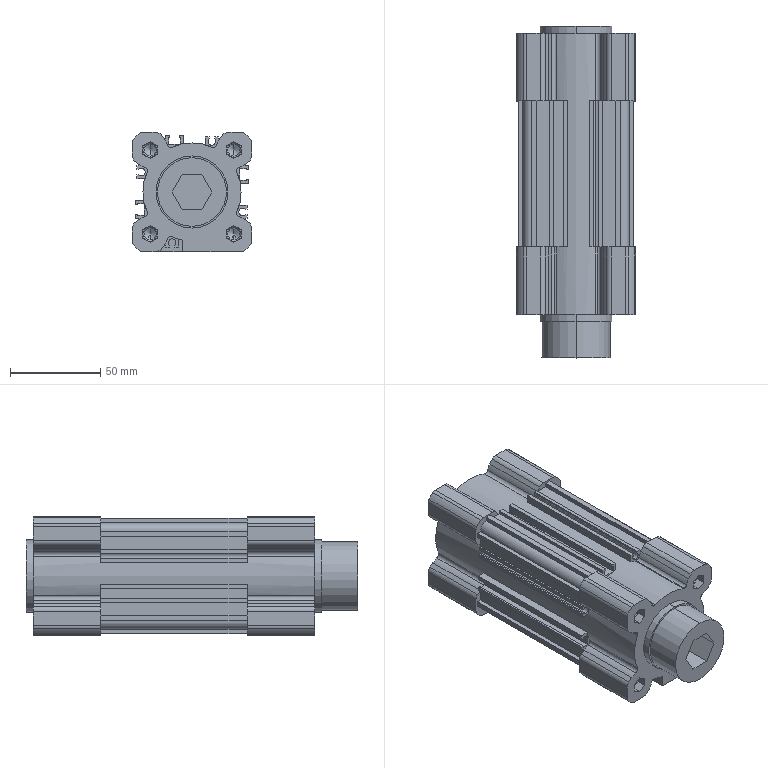Part | SolidWorks | features BaseBody 1 | 1 solid | 407 faces | box 66 x 184 x 66 mm | volume 428858 mm3 | plane 263 | cylinder 112 | cone 32 | commonest cylinder face diameters 7 x30 4 x17 6.647 x16 20 x14 4.25 x9 22 x8